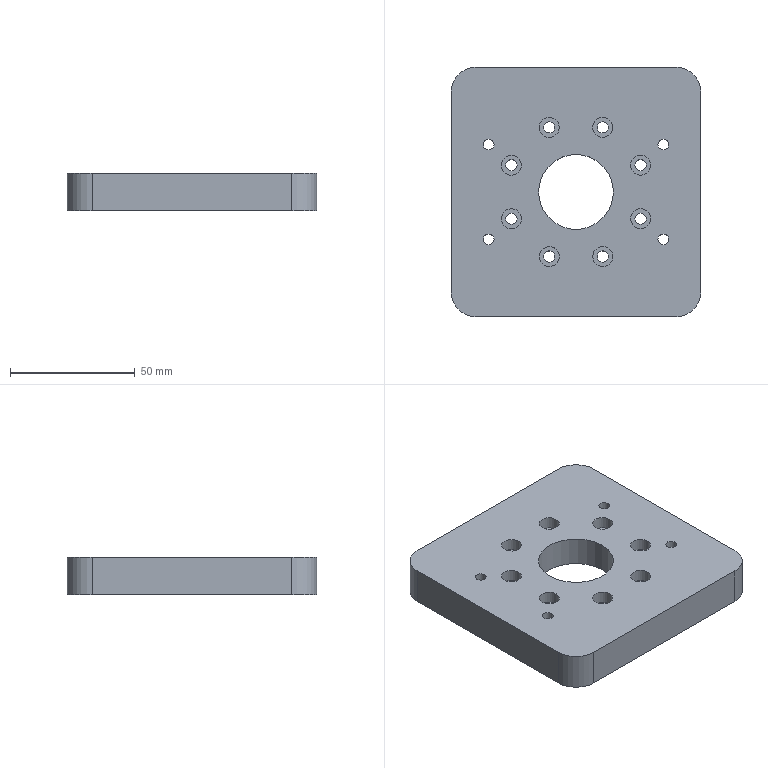NC program | NX | posted with a generic post | part box 100 x 100 x 15 mm
Lines 25 to 866 of 2115:
(ZLEVEL_PROFILE , TOOL : D10)
N48 T10 M6
N50 G54
N52 G17 G0 G90 X-53.178 Y-47.366 S9500 M3
N54 G43 Z30. H10
N56 Z1.5
N58 G94 G1 X-54.028 Y-45.669 Z1.401 F1000.
N60 X-54.754 Y-43.354 Z1.273
N62 X-55.1 Y-40.952 Z1.146
N64 Y-40. Z1.096
N66 Y0. Z-1.
N68 Y40. F3500.
N70 G2 X-40. Y55.1 R15.1
N72 G1 X40.
N74 G2 X55.1 Y40. R15.1
N76 G1 Y-40.
N78 G2 X40. Y-55.1 R15.1
N80 G1 X-40.
N82 G2 X-55.1 Y-40. R15.1
N84 G1 Y0.
N86 Y30. Z-1.072
N88 Y35. Z-1.084
N90 Y40. Z-1.096
N92 X-55.072 Y40.912 Z-1.099
N94 X-54.99 Y41.82 Z-1.101
N96 X-54.853 Y42.722 Z-1.103
N98 X-54.661 Y43.614 Z-1.105
N100 X-54.416 Y44.492 Z-1.107
N102 X-54.119 Y45.355 Z-1.11
N104 X-53.77 Y46.197 Z-1.112
N106 X-53.37 Y47.017 Z-1.114
N108 X-52.922 Y47.812 Z-1.116
N110 X-52.427 Y48.578 Z-1.118
N112 X-51.886 Y49.312 Z-1.121
N114 X-51.303 Y50.013 Z-1.123
N116 X-50.677 Y50.677 Z-1.125
N118 X-50.013 Y51.303 Z-1.127
N120 X-49.312 Y51.886 Z-1.129
N122 X-48.578 Y52.427 Z-1.132
N124 X-47.812 Y52.922 Z-1.134
N126 X-47.017 Y53.37 Z-1.136
N128 X-46.197 Y53.77 Z-1.138
N130 X-45.355 Y54.119 Z-1.14
N132 X-44.492 Y54.416 Z-1.143
N134 X-43.614 Y54.661 Z-1.145
N136 X-42.722 Y54.853 Z-1.147
N138 X-41.82 Y54.99 Z-1.149
N140 X-40.912 Y55.072 Z-1.151
N142 X-40. Y55.1 Z-1.154
N144 X30. Z-1.322
N146 X35. Z-1.334
N148 X40. Z-1.346
N150 X40.912 Y55.072 Z-1.349
N152 X41.82 Y54.99 Z-1.351
N154 X42.722 Y54.853 Z-1.353
N156 X43.614 Y54.661 Z-1.355
N158 X44.492 Y54.416 Z-1.357
N160 X45.355 Y54.119 Z-1.36
N162 X46.197 Y53.77 Z-1.362
N164 X47.017 Y53.37 Z-1.364
N166 X47.812 Y52.922 Z-1.366
N168 X48.578 Y52.427 Z-1.368
N170 X49.312 Y51.886 Z-1.371
N172 X50.013 Y51.303 Z-1.373
N174 X50.677 Y50.677 Z-1.375
N176 X51.303 Y50.013 Z-1.377
N178 X51.886 Y49.312 Z-1.379
N180 X52.427 Y48.578 Z-1.382
N182 X52.922 Y47.812 Z-1.384
N184 X53.37 Y47.017 Z-1.386
N186 X53.77 Y46.197 Z-1.388
N188 X54.119 Y45.355 Z-1.39
N190 X54.416 Y44.492 Z-1.393
N192 X54.661 Y43.614 Z-1.395
N194 X54.853 Y42.722 Z-1.397
N196 X54.99 Y41.82 Z-1.399
N198 X55.072 Y40.912 Z-1.401
N200 X55.1 Y40. Z-1.404
N202 Y-40. Z-1.596
N204 X55.072 Y-40.912 Z-1.599
N206 X54.99 Y-41.82 Z-1.601
N208 X54.853 Y-42.722 Z-1.603
N210 X54.661 Y-43.614 Z-1.605
N212 X54.416 Y-44.492 Z-1.607
N214 X54.119 Y-45.355 Z-1.61
N216 X53.77 Y-46.197 Z-1.612
N218 X53.37 Y-47.017 Z-1.614
N220 X52.922 Y-47.812 Z-1.616
N222 X52.427 Y-48.578 Z-1.618
N224 X51.886 Y-49.312 Z-1.621
N226 X51.303 Y-50.013 Z-1.623
N228 X50.677 Y-50.677 Z-1.625
N230 X50.013 Y-51.303 Z-1.627
N232 X49.312 Y-51.886 Z-1.629
N234 X48.578 Y-52.427 Z-1.632
N236 X47.812 Y-52.922 Z-1.634
N238 X47.017 Y-53.37 Z-1.636
N240 X46.197 Y-53.77 Z-1.638
N242 X45.355 Y-54.119 Z-1.64
N244 X44.492 Y-54.416 Z-1.643
N246 X43.614 Y-54.661 Z-1.645
N248 X42.722 Y-54.853 Z-1.647
N250 X41.82 Y-54.99 Z-1.649
N252 X40.912 Y-55.072 Z-1.651
N254 X40. Y-55.1 Z-1.654
N256 X-30. Z-1.822
N258 X-35. Z-1.834
N260 X-40. Z-1.846
N262 X-40.912 Y-55.072 Z-1.849
N264 X-41.82 Y-54.99 Z-1.851
N266 X-42.722 Y-54.853 Z-1.853
N268 X-43.614 Y-54.661 Z-1.855
N270 X-44.492 Y-54.416 Z-1.857
N272 X-45.355 Y-54.119 Z-1.86
N274 X-46.197 Y-53.77 Z-1.862
N276 X-47.017 Y-53.37 Z-1.864
N278 X-47.812 Y-52.922 Z-1.866
N280 X-48.578 Y-52.427 Z-1.868
N282 X-49.312 Y-51.886 Z-1.871
N284 X-50.013 Y-51.303 Z-1.873
N286 X-50.677 Y-50.677 Z-1.875
N288 X-51.303 Y-50.013 Z-1.877
N290 X-51.886 Y-49.312 Z-1.879
N292 X-52.427 Y-48.578 Z-1.882
N294 X-52.922 Y-47.812 Z-1.884
N296 X-53.37 Y-47.017 Z-1.886
N298 X-53.77 Y-46.197 Z-1.888
N300 X-54.119 Y-45.355 Z-1.89
N302 X-54.416 Y-44.492 Z-1.893
N304 X-54.661 Y-43.614 Z-1.895
N306 X-54.853 Y-42.722 Z-1.897
N308 X-54.99 Y-41.82 Z-1.899
N310 X-55.072 Y-40.912 Z-1.901
N312 X-55.1 Y-40. Z-1.904
N314 Y0. Z-2.
N316 Y30. Z-2.072
N318 Y35. Z-2.084
N320 Y40. Z-2.096
N322 X-55.072 Y40.912 Z-2.099
N324 X-54.99 Y41.82 Z-2.101
N326 X-54.853 Y42.722 Z-2.103
N328 X-54.661 Y43.614 Z-2.105
N330 X-54.416 Y44.492 Z-2.107
N332 X-54.119 Y45.355 Z-2.11
N334 X-53.77 Y46.197 Z-2.112
N336 X-53.37 Y47.017 Z-2.114
N338 X-52.922 Y47.812 Z-2.116
N340 X-52.427 Y48.578 Z-2.118
N342 X-51.886 Y49.312 Z-2.121
N344 X-51.303 Y50.013 Z-2.123
N346 X-50.677 Y50.677 Z-2.125
N348 X-50.013 Y51.303 Z-2.127
N350 X-49.312 Y51.886 Z-2.129
N352 X-48.578 Y52.427 Z-2.132
N354 X-47.812 Y52.922 Z-2.134
N356 X-47.017 Y53.37 Z-2.136
N358 X-46.197 Y53.77 Z-2.138
N360 X-45.355 Y54.119 Z-2.14
N362 X-44.492 Y54.416 Z-2.143
N364 X-43.614 Y54.661 Z-2.145
N366 X-42.722 Y54.853 Z-2.147
N368 X-41.82 Y54.99 Z-2.149
N370 X-40.912 Y55.072 Z-2.151
N372 X-40. Y55.1 Z-2.154
N374 X30. Z-2.322
N376 X35. Z-2.334
N378 X40. Z-2.346
N380 X40.912 Y55.072 Z-2.349
N382 X41.82 Y54.99 Z-2.351
N384 X42.722 Y54.853 Z-2.353
N386 X43.614 Y54.661 Z-2.355
N388 X44.492 Y54.416 Z-2.357
N390 X45.355 Y54.119 Z-2.36
N392 X46.197 Y53.77 Z-2.362
N394 X47.017 Y53.37 Z-2.364
N396 X47.812 Y52.922 Z-2.366
N398 X48.578 Y52.427 Z-2.368
N400 X49.312 Y51.886 Z-2.371
N402 X50.013 Y51.303 Z-2.373
N404 X50.677 Y50.677 Z-2.375
N406 X51.303 Y50.013 Z-2.377
N408 X51.886 Y49.312 Z-2.379
N410 X52.427 Y48.578 Z-2.382
N412 X52.922 Y47.812 Z-2.384
N414 X53.37 Y47.017 Z-2.386
N416 X53.77 Y46.197 Z-2.388
N418 X54.119 Y45.355 Z-2.39
N420 X54.416 Y44.492 Z-2.393
N422 X54.661 Y43.614 Z-2.395
N424 X54.853 Y42.722 Z-2.397
N426 X54.99 Y41.82 Z-2.399
N428 X55.072 Y40.912 Z-2.401
N430 X55.1 Y40. Z-2.404
N432 Y-40. Z-2.596
N434 X55.072 Y-40.912 Z-2.599
N436 X54.99 Y-41.82 Z-2.601
N438 X54.853 Y-42.722 Z-2.603
N440 X54.661 Y-43.614 Z-2.605
N442 X54.416 Y-44.492 Z-2.607
N444 X54.119 Y-45.355 Z-2.61
N446 X53.77 Y-46.197 Z-2.612
N448 X53.37 Y-47.017 Z-2.614
N450 X52.922 Y-47.812 Z-2.616
N452 X52.427 Y-48.578 Z-2.618
N454 X51.886 Y-49.312 Z-2.621
N456 X51.303 Y-50.013 Z-2.623
N458 X50.677 Y-50.677 Z-2.625
N460 X50.013 Y-51.303 Z-2.627
N462 X49.312 Y-51.886 Z-2.629
N464 X48.578 Y-52.427 Z-2.632
N466 X47.812 Y-52.922 Z-2.634
N468 X47.017 Y-53.37 Z-2.636
N470 X46.197 Y-53.77 Z-2.638
N472 X45.355 Y-54.119 Z-2.64
N474 X44.492 Y-54.416 Z-2.643
N476 X43.614 Y-54.661 Z-2.645
N478 X42.722 Y-54.853 Z-2.647
N480 X41.82 Y-54.99 Z-2.649
N482 X40.912 Y-55.072 Z-2.651
N484 X40. Y-55.1 Z-2.654
N486 X-30. Z-2.822
N488 X-35. Z-2.834
N490 X-40. Z-2.846
N492 X-40.912 Y-55.072 Z-2.849
N494 X-41.82 Y-54.99 Z-2.851
N496 X-42.722 Y-54.853 Z-2.853
N498 X-43.614 Y-54.661 Z-2.855
N500 X-44.492 Y-54.416 Z-2.857
N502 X-45.355 Y-54.119 Z-2.86
N504 X-46.197 Y-53.77 Z-2.862
N506 X-47.017 Y-53.37 Z-2.864
N508 X-47.812 Y-52.922 Z-2.866
N510 X-48.578 Y-52.427 Z-2.868
N512 X-49.312 Y-51.886 Z-2.871
N514 X-50.013 Y-51.303 Z-2.873
N516 X-50.677 Y-50.677 Z-2.875
N518 X-51.303 Y-50.013 Z-2.877
N520 X-51.886 Y-49.312 Z-2.879
N522 X-52.427 Y-48.578 Z-2.882
N524 X-52.922 Y-47.812 Z-2.884
N526 X-53.37 Y-47.017 Z-2.886
N528 X-53.77 Y-46.197 Z-2.888
N530 X-54.119 Y-45.355 Z-2.89
N532 X-54.416 Y-44.492 Z-2.893
N534 X-54.661 Y-43.614 Z-2.895
N536 X-54.853 Y-42.722 Z-2.897
N538 X-54.99 Y-41.82 Z-2.899
N540 X-55.072 Y-40.912 Z-2.901
N542 X-55.1 Y-40. Z-2.904
N544 Y0. Z-3.
N546 Y30. Z-3.072
N548 Y35. Z-3.084
N550 Y40. Z-3.096
N552 X-55.072 Y40.912 Z-3.099
N554 X-54.99 Y41.82 Z-3.101
N556 X-54.853 Y42.722 Z-3.103
N558 X-54.661 Y43.614 Z-3.105
N560 X-54.416 Y44.492 Z-3.107
N562 X-54.119 Y45.355 Z-3.11
N564 X-53.77 Y46.197 Z-3.112
N566 X-53.37 Y47.017 Z-3.114
N568 X-52.922 Y47.812 Z-3.116
N570 X-52.427 Y48.578 Z-3.118
N572 X-51.886 Y49.312 Z-3.121
N574 X-51.303 Y50.013 Z-3.123
N576 X-50.677 Y50.677 Z-3.125
N578 X-50.013 Y51.303 Z-3.127
N580 X-49.312 Y51.886 Z-3.129
N582 X-48.578 Y52.427 Z-3.132
N584 X-47.812 Y52.922 Z-3.134
N586 X-47.017 Y53.37 Z-3.136
N588 X-46.197 Y53.77 Z-3.138
N590 X-45.355 Y54.119 Z-3.14
N592 X-44.492 Y54.416 Z-3.143
N594 X-43.614 Y54.661 Z-3.145
N596 X-42.722 Y54.853 Z-3.147
N598 X-41.82 Y54.99 Z-3.149
N600 X-40.912 Y55.072 Z-3.151
N602 X-40. Y55.1 Z-3.154
N604 X30. Z-3.322
N606 X35. Z-3.334
N608 X40. Z-3.346
N610 X40.912 Y55.072 Z-3.349
N612 X41.82 Y54.99 Z-3.351
N614 X42.722 Y54.853 Z-3.353
N616 X43.614 Y54.661 Z-3.355
N618 X44.492 Y54.416 Z-3.357
N620 X45.355 Y54.119 Z-3.36
N622 X46.197 Y53.77 Z-3.362
N624 X47.017 Y53.37 Z-3.364
N626 X47.812 Y52.922 Z-3.366
N628 X48.578 Y52.427 Z-3.368
N630 X49.312 Y51.886 Z-3.371
N632 X50.013 Y51.303 Z-3.373
N634 X50.677 Y50.677 Z-3.375
N636 X51.303 Y50.013 Z-3.377
N638 X51.886 Y49.312 Z-3.379
N640 X52.427 Y48.578 Z-3.382
N642 X52.922 Y47.812 Z-3.384
N644 X53.37 Y47.017 Z-3.386
N646 X53.77 Y46.197 Z-3.388
N648 X54.119 Y45.355 Z-3.39
N650 X54.416 Y44.492 Z-3.393
N652 X54.661 Y43.614 Z-3.395
N654 X54.853 Y42.722 Z-3.397
N656 X54.99 Y41.82 Z-3.399
N658 X55.072 Y40.912 Z-3.401
N660 X55.1 Y40. Z-3.404
N662 Y-40. Z-3.596
N664 X55.072 Y-40.912 Z-3.599
N666 X54.99 Y-41.82 Z-3.601
N668 X54.853 Y-42.722 Z-3.603
N670 X54.661 Y-43.614 Z-3.605
N672 X54.416 Y-44.492 Z-3.607
N674 X54.119 Y-45.355 Z-3.61
N676 X53.77 Y-46.197 Z-3.612
N678 X53.37 Y-47.017 Z-3.614
N680 X52.922 Y-47.812 Z-3.616
N682 X52.427 Y-48.578 Z-3.618
N684 X51.886 Y-49.312 Z-3.621
N686 X51.303 Y-50.013 Z-3.623
N688 X50.677 Y-50.677 Z-3.625
N690 X50.013 Y-51.303 Z-3.627
N692 X49.312 Y-51.886 Z-3.629
N694 X48.578 Y-52.427 Z-3.632
N696 X47.812 Y-52.922 Z-3.634
N698 X47.017 Y-53.37 Z-3.636
N700 X46.197 Y-53.77 Z-3.638
N702 X45.355 Y-54.119 Z-3.64
N704 X44.492 Y-54.416 Z-3.643
N706 X43.614 Y-54.661 Z-3.645
N708 X42.722 Y-54.853 Z-3.647
N710 X41.82 Y-54.99 Z-3.649
N712 X40.912 Y-55.072 Z-3.651
N714 X40. Y-55.1 Z-3.654
N716 X-30. Z-3.822
N718 X-35. Z-3.834
N720 X-40. Z-3.846
N722 X-40.912 Y-55.072 Z-3.849
N724 X-41.82 Y-54.99 Z-3.851
N726 X-42.722 Y-54.853 Z-3.853
N728 X-43.614 Y-54.661 Z-3.855
N730 X-44.492 Y-54.416 Z-3.857
N732 X-45.355 Y-54.119 Z-3.86
N734 X-46.197 Y-53.77 Z-3.862
N736 X-47.017 Y-53.37 Z-3.864
N738 X-47.812 Y-52.922 Z-3.866
N740 X-48.578 Y-52.427 Z-3.868
N742 X-49.312 Y-51.886 Z-3.871
N744 X-50.013 Y-51.303 Z-3.873
N746 X-50.677 Y-50.677 Z-3.875
N748 X-51.303 Y-50.013 Z-3.877
N750 X-51.886 Y-49.312 Z-3.879
N752 X-52.427 Y-48.578 Z-3.882
N754 X-52.922 Y-47.812 Z-3.884
N756 X-53.37 Y-47.017 Z-3.886
N758 X-53.77 Y-46.197 Z-3.888
N760 X-54.119 Y-45.355 Z-3.89
N762 X-54.416 Y-44.492 Z-3.893
N764 X-54.661 Y-43.614 Z-3.895
N766 X-54.853 Y-42.722 Z-3.897
N768 X-54.99 Y-41.82 Z-3.899
N770 X-55.072 Y-40.912 Z-3.901
N772 X-55.1 Y-40. Z-3.904
N774 Y0. Z-4.
N776 Y30. Z-4.072
N778 Y35. Z-4.084
N780 Y40. Z-4.096
N782 X-55.072 Y40.912 Z-4.099
N784 X-54.99 Y41.82 Z-4.101
N786 X-54.853 Y42.722 Z-4.103
N788 X-54.661 Y43.614 Z-4.105
N790 X-54.416 Y44.492 Z-4.107
N792 X-54.119 Y45.355 Z-4.11
N794 X-53.77 Y46.197 Z-4.112
N796 X-53.37 Y47.017 Z-4.114
N798 X-52.922 Y47.812 Z-4.116
N800 X-52.427 Y48.578 Z-4.118
N802 X-51.886 Y49.312 Z-4.121
N804 X-51.303 Y50.013 Z-4.123
N806 X-50.677 Y50.677 Z-4.125
N808 X-50.013 Y51.303 Z-4.127
N810 X-49.312 Y51.886 Z-4.129
N812 X-48.578 Y52.427 Z-4.132
N814 X-47.812 Y52.922 Z-4.134
N816 X-47.017 Y53.37 Z-4.136
N818 X-46.197 Y53.77 Z-4.138
N820 X-45.355 Y54.119 Z-4.14
N822 X-44.492 Y54.416 Z-4.143
N824 X-43.614 Y54.661 Z-4.145
N826 X-42.722 Y54.853 Z-4.147
N828 X-41.82 Y54.99 Z-4.149
N830 X-40.912 Y55.072 Z-4.151
N832 X-40. Y55.1 Z-4.154
N834 X30. Z-4.322
N836 X35. Z-4.334
N838 X40. Z-4.346
N840 X40.912 Y55.072 Z-4.349
N842 X41.82 Y54.99 Z-4.351
N844 X42.722 Y54.853 Z-4.353
N846 X43.614 Y54.661 Z-4.355
N848 X44.492 Y54.416 Z-4.357
N850 X45.355 Y54.119 Z-4.36
N852 X46.197 Y53.77 Z-4.362
N854 X47.017 Y53.37 Z-4.364
N856 X47.812 Y52.922 Z-4.366
N858 X48.578 Y52.427 Z-4.368
N860 X49.312 Y51.886 Z-4.371
N862 X50.013 Y51.303 Z-4.373
N864 X50.677 Y50.677 Z-4.375
N866 X51.303 Y50.013 Z-4.377
N868 X51.886 Y49.312 Z-4.379
N870 X52.427 Y48.578 Z-4.382
N872 X52.922 Y47.812 Z-4.384
N874 X53.37 Y47.017 Z-4.386
N876 X53.77 Y46.197 Z-4.388
N878 X54.119 Y45.355 Z-4.39
N880 X54.416 Y44.492 Z-4.393
N882 X54.661 Y43.614 Z-4.395
N884 X54.853 Y42.722 Z-4.397
N886 X54.99 Y41.82 Z-4.399
N888 X55.072 Y40.912 Z-4.401
N890 X55.1 Y40. Z-4.404
N892 Y-40. Z-4.596
N894 X55.072 Y-40.912 Z-4.599
N896 X54.99 Y-41.82 Z-4.601
N898 X54.853 Y-42.722 Z-4.603
N900 X54.661 Y-43.614 Z-4.605
N902 X54.416 Y-44.492 Z-4.607
N904 X54.119 Y-45.355 Z-4.61
N906 X53.77 Y-46.197 Z-4.612
N908 X53.37 Y-47.017 Z-4.614
N910 X52.922 Y-47.812 Z-4.616
N912 X52.427 Y-48.578 Z-4.618
N914 X51.886 Y-49.312 Z-4.621
N916 X51.303 Y-50.013 Z-4.623
N918 X50.677 Y-50.677 Z-4.625
N920 X50.013 Y-51.303 Z-4.627
N922 X49.312 Y-51.886 Z-4.629
N924 X48.578 Y-52.427 Z-4.632
N926 X47.812 Y-52.922 Z-4.634
N928 X47.017 Y-53.37 Z-4.636
N930 X46.197 Y-53.77 Z-4.638
N932 X45.355 Y-54.119 Z-4.64
N934 X44.492 Y-54.416 Z-4.643
N936 X43.614 Y-54.661 Z-4.645
N938 X42.722 Y-54.853 Z-4.647
N940 X41.82 Y-54.99 Z-4.649
N942 X40.912 Y-55.072 Z-4.651
N944 X40. Y-55.1 Z-4.654
N946 X-30. Z-4.822
N948 X-35. Z-4.834
N950 X-40. Z-4.846
N952 X-40.912 Y-55.072 Z-4.849
N954 X-41.82 Y-54.99 Z-4.851
N956 X-42.722 Y-54.853 Z-4.853
N958 X-43.614 Y-54.661 Z-4.855
N960 X-44.492 Y-54.416 Z-4.857
N962 X-45.355 Y-54.119 Z-4.86
N964 X-46.197 Y-53.77 Z-4.862
N966 X-47.017 Y-53.37 Z-4.864
N968 X-47.812 Y-52.922 Z-4.866
N970 X-48.578 Y-52.427 Z-4.868
N972 X-49.312 Y-51.886 Z-4.871
N974 X-50.013 Y-51.303 Z-4.873
N976 X-50.677 Y-50.677 Z-4.875
N978 X-51.303 Y-50.013 Z-4.877
N980 X-51.886 Y-49.312 Z-4.879
N982 X-52.427 Y-48.578 Z-4.882
N984 X-52.922 Y-47.812 Z-4.884
N986 X-53.37 Y-47.017 Z-4.886
N988 X-53.77 Y-46.197 Z-4.888
N990 X-54.119 Y-45.355 Z-4.89
N992 X-54.416 Y-44.492 Z-4.893
N994 X-54.661 Y-43.614 Z-4.895
N996 X-54.853 Y-42.722 Z-4.897
N998 X-54.99 Y-41.82 Z-4.899
N1000 X-55.072 Y-40.912 Z-4.901
N1002 X-55.1 Y-40. Z-4.904
N1004 Y0. Z-5.
N1006 Y30. Z-5.072
N1008 Y35. Z-5.084
N1010 Y40. Z-5.096
N1012 X-55.072 Y40.912 Z-5.099
N1014 X-54.99 Y41.82 Z-5.101
N1016 X-54.853 Y42.722 Z-5.103
N1018 X-54.661 Y43.614 Z-5.105
N1020 X-54.416 Y44.492 Z-5.107
N1022 X-54.119 Y45.355 Z-5.11
N1024 X-53.77 Y46.197 Z-5.112
N1026 X-53.37 Y47.017 Z-5.114
N1028 X-52.922 Y47.812 Z-5.116
N1030 X-52.427 Y48.578 Z-5.118
N1032 X-51.886 Y49.312 Z-5.121
N1034 X-51.303 Y50.013 Z-5.123
N1036 X-50.677 Y50.677 Z-5.125
N1038 X-50.013 Y51.303 Z-5.127
N1040 X-49.312 Y51.886 Z-5.129
N1042 X-48.578 Y52.427 Z-5.132
N1044 X-47.812 Y52.922 Z-5.134
N1046 X-47.017 Y53.37 Z-5.136
N1048 X-46.197 Y53.77 Z-5.138
N1050 X-45.355 Y54.119 Z-5.14
N1052 X-44.492 Y54.416 Z-5.143
N1054 X-43.614 Y54.661 Z-5.145
N1056 X-42.722 Y54.853 Z-5.147
N1058 X-41.82 Y54.99 Z-5.149
N1060 X-40.912 Y55.072 Z-5.151
N1062 X-40. Y55.1 Z-5.154
N1064 X30. Z-5.322
N1066 X35. Z-5.334
N1068 X40. Z-5.346
N1070 X40.912 Y55.072 Z-5.349
N1072 X41.82 Y54.99 Z-5.351
N1074 X42.722 Y54.853 Z-5.353
N1076 X43.614 Y54.661 Z-5.355
N1078 X44.492 Y54.416 Z-5.357
N1080 X45.355 Y54.119 Z-5.36
N1082 X46.197 Y53.77 Z-5.362
N1084 X47.017 Y53.37 Z-5.364
N1086 X47.812 Y52.922 Z-5.366
N1088 X48.578 Y52.427 Z-5.368
N1090 X49.312 Y51.886 Z-5.371
N1092 X50.013 Y51.303 Z-5.373
N1094 X50.677 Y50.677 Z-5.375
N1096 X51.303 Y50.013 Z-5.377
N1098 X51.886 Y49.312 Z-5.379
N1100 X52.427 Y48.578 Z-5.382
N1102 X52.922 Y47.812 Z-5.384
N1104 X53.37 Y47.017 Z-5.386
N1106 X53.77 Y46.197 Z-5.388
N1108 X54.119 Y45.355 Z-5.39
N1110 X54.416 Y44.492 Z-5.393
N1112 X54.661 Y43.614 Z-5.395
N1114 X54.853 Y42.722 Z-5.397
N1116 X54.99 Y41.82 Z-5.399
N1118 X55.072 Y40.912 Z-5.401
N1120 X55.1 Y40. Z-5.404
N1122 Y-40. Z-5.596
N1124 X55.072 Y-40.912 Z-5.599
N1126 X54.99 Y-41.82 Z-5.601
N1128 X54.853 Y-42.722 Z-5.603
N1130 X54.661 Y-43.614 Z-5.605
N1132 X54.416 Y-44.492 Z-5.607
N1134 X54.119 Y-45.355 Z-5.61
N1136 X53.77 Y-46.197 Z-5.612
N1138 X53.37 Y-47.017 Z-5.614
N1140 X52.922 Y-47.812 Z-5.616
N1142 X52.427 Y-48.578 Z-5.618
N1144 X51.886 Y-49.312 Z-5.621
N1146 X51.303 Y-50.013 Z-5.623
N1148 X50.677 Y-50.677 Z-5.625
N1150 X50.013 Y-51.303 Z-5.627
N1152 X49.312 Y-51.886 Z-5.629
N1154 X48.578 Y-52.427 Z-5.632
N1156 X47.812 Y-52.922 Z-5.634
N1158 X47.017 Y-53.37 Z-5.636
N1160 X46.197 Y-53.77 Z-5.638
N1162 X45.355 Y-54.119 Z-5.64
N1164 X44.492 Y-54.416 Z-5.643
N1166 X43.614 Y-54.661 Z-5.645
N1168 X42.722 Y-54.853 Z-5.647
N1170 X41.82 Y-54.99 Z-5.649
N1172 X40.912 Y-55.072 Z-5.651
N1174 X40. Y-55.1 Z-5.654
N1176 X-30. Z-5.822
N1178 X-35. Z-5.834
N1180 X-40. Z-5.846
N1182 X-40.912 Y-55.072 Z-5.849
N1184 X-41.82 Y-54.99 Z-5.851
N1186 X-42.722 Y-54.853 Z-5.853
N1188 X-43.614 Y-54.661 Z-5.855
N1190 X-44.492 Y-54.416 Z-5.857
N1192 X-45.355 Y-54.119 Z-5.86
N1194 X-46.197 Y-53.77 Z-5.862
N1196 X-47.017 Y-53.37 Z-5.864
N1198 X-47.812 Y-52.922 Z-5.866
N1200 X-48.578 Y-52.427 Z-5.868
N1202 X-49.312 Y-51.886 Z-5.871
N1204 X-50.013 Y-51.303 Z-5.873
N1206 X-50.677 Y-50.677 Z-5.875
N1208 X-51.303 Y-50.013 Z-5.877
N1210 X-51.886 Y-49.312 Z-5.879
N1212 X-52.427 Y-48.578 Z-5.882
N1214 X-52.922 Y-47.812 Z-5.884
N1216 X-53.37 Y-47.017 Z-5.886
N1218 X-53.77 Y-46.197 Z-5.888
N1220 X-54.119 Y-45.355 Z-5.89
N1222 X-54.416 Y-44.492 Z-5.893
N1224 X-54.661 Y-43.614 Z-5.895
N1226 X-54.853 Y-42.722 Z-5.897
N1228 X-54.99 Y-41.82 Z-5.899
N1230 X-55.072 Y-40.912 Z-5.901
N1232 X-55.1 Y-40. Z-5.904
N1234 Y0. Z-6.
N1236 Y30. Z-6.072
N1238 Y35. Z-6.084
N1240 Y40. Z-6.096
N1242 X-55.072 Y40.912 Z-6.099
N1244 X-54.99 Y41.82 Z-6.101
N1246 X-54.853 Y42.722 Z-6.103
N1248 X-54.661 Y43.614 Z-6.105
N1250 X-54.416 Y44.492 Z-6.107
N1252 X-54.119 Y45.355 Z-6.11
N1254 X-53.77 Y46.197 Z-6.112
N1256 X-53.37 Y47.017 Z-6.114
N1258 X-52.922 Y47.812 Z-6.116
N1260 X-52.427 Y48.578 Z-6.118
N1262 X-51.886 Y49.312 Z-6.121
N1264 X-51.303 Y50.013 Z-6.123
N1266 X-50.677 Y50.677 Z-6.125
N1268 X-50.013 Y51.303 Z-6.127
N1270 X-49.312 Y51.886 Z-6.129
N1272 X-48.578 Y52.427 Z-6.132
N1274 X-47.812 Y52.922 Z-6.134
N1276 X-47.017 Y53.37 Z-6.136
N1278 X-46.197 Y53.77 Z-6.138
N1280 X-45.355 Y54.119 Z-6.14
N1282 X-44.492 Y54.416 Z-6.143
N1284 X-43.614 Y54.661 Z-6.145
N1286 X-42.722 Y54.853 Z-6.147
N1288 X-41.82 Y54.99 Z-6.149
N1290 X-40.912 Y55.072 Z-6.151
N1292 X-40. Y55.1 Z-6.154
N1294 X30. Z-6.322
N1296 X35. Z-6.334
N1298 X40. Z-6.346
N1300 X40.912 Y55.072 Z-6.349
N1302 X41.82 Y54.99 Z-6.351
N1304 X42.722 Y54.853 Z-6.353
N1306 X43.614 Y54.661 Z-6.355
N1308 X44.492 Y54.416 Z-6.357
N1310 X45.355 Y54.119 Z-6.36
N1312 X46.197 Y53.77 Z-6.362
N1314 X47.017 Y53.37 Z-6.364
N1316 X47.812 Y52.922 Z-6.366
N1318 X48.578 Y52.427 Z-6.368
N1320 X49.312 Y51.886 Z-6.371
N1322 X50.013 Y51.303 Z-6.373
N1324 X50.677 Y50.677 Z-6.375
N1326 X51.303 Y50.013 Z-6.377
N1328 X51.886 Y49.312 Z-6.379
N1330 X52.427 Y48.578 Z-6.382
N1332 X52.922 Y47.812 Z-6.384
N1334 X53.37 Y47.017 Z-6.386
N1336 X53.77 Y46.197 Z-6.388
N1338 X54.119 Y45.355 Z-6.39
N1340 X54.416 Y44.492 Z-6.393
N1342 X54.661 Y43.614 Z-6.395
N1344 X54.853 Y42.722 Z-6.397
N1346 X54.99 Y41.82 Z-6.399
N1348 X55.072 Y40.912 Z-6.401
N1350 X55.1 Y40. Z-6.404
N1352 Y-40. Z-6.596
N1354 X55.072 Y-40.912 Z-6.599
N1356 X54.99 Y-41.82 Z-6.601
N1358 X54.853 Y-42.722 Z-6.603
N1360 X54.661 Y-43.614 Z-6.605
N1362 X54.416 Y-44.492 Z-6.607
N1364 X54.119 Y-45.355 Z-6.61
N1366 X53.77 Y-46.197 Z-6.612
N1368 X53.37 Y-47.017 Z-6.614
N1370 X52.922 Y-47.812 Z-6.616
N1372 X52.427 Y-48.578 Z-6.618
N1374 X51.886 Y-49.312 Z-6.621
N1376 X51.303 Y-50.013 Z-6.623
N1378 X50.677 Y-50.677 Z-6.625
N1380 X50.013 Y-51.303 Z-6.627
N1382 X49.312 Y-51.886 Z-6.629
N1384 X48.578 Y-52.427 Z-6.632
N1386 X47.812 Y-52.922 Z-6.634
N1388 X47.017 Y-53.37 Z-6.636
N1390 X46.197 Y-53.77 Z-6.638
N1392 X45.355 Y-54.119 Z-6.64
N1394 X44.492 Y-54.416 Z-6.643
N1396 X43.614 Y-54.661 Z-6.645
N1398 X42.722 Y-54.853 Z-6.647
N1400 X41.82 Y-54.99 Z-6.649
N1402 X40.912 Y-55.072 Z-6.651
N1404 X40. Y-55.1 Z-6.654
N1406 X-30. Z-6.822
N1408 X-35. Z-6.834
N1410 X-40. Z-6.846
N1412 X-40.912 Y-55.072 Z-6.849
N1414 X-41.82 Y-54.99 Z-6.851
N1416 X-42.722 Y-54.853 Z-6.853
N1418 X-43.614 Y-54.661 Z-6.855
N1420 X-44.492 Y-54.416 Z-6.857
N1422 X-45.355 Y-54.119 Z-6.86
N1424 X-46.197 Y-53.77 Z-6.862
N1426 X-47.017 Y-53.37 Z-6.864
N1428 X-47.812 Y-52.922 Z-6.866
N1430 X-48.578 Y-52.427 Z-6.868
N1432 X-49.312 Y-51.886 Z-6.871
N1434 X-50.013 Y-51.303 Z-6.873
N1436 X-50.677 Y-50.677 Z-6.875
N1438 X-51.303 Y-50.013 Z-6.877
N1440 X-51.886 Y-49.312 Z-6.879
N1442 X-52.427 Y-48.578 Z-6.882
N1444 X-52.922 Y-47.812 Z-6.884
N1446 X-53.37 Y-47.017 Z-6.886
N1448 X-53.77 Y-46.197 Z-6.888
N1450 X-54.119 Y-45.355 Z-6.89
N1452 X-54.416 Y-44.492 Z-6.893
N1454 X-54.661 Y-43.614 Z-6.895
N1456 X-54.853 Y-42.722 Z-6.897
N1458 X-54.99 Y-41.82 Z-6.899
N1460 X-55.072 Y-40.912 Z-6.901
N1462 X-55.1 Y-40. Z-6.904
N1464 Y0. Z-7.
N1466 Y30. Z-7.072
N1468 Y35. Z-7.084
N1470 Y40. Z-7.096
N1472 X-55.072 Y40.912 Z-7.099
N1474 X-54.99 Y41.82 Z-7.101
N1476 X-54.853 Y42.722 Z-7.103
N1478 X-54.661 Y43.614 Z-7.105
N1480 X-54.416 Y44.492 Z-7.107
N1482 X-54.119 Y45.355 Z-7.11
N1484 X-53.77 Y46.197 Z-7.112
N1486 X-53.37 Y47.017 Z-7.114
N1488 X-52.922 Y47.812 Z-7.116
N1490 X-52.427 Y48.578 Z-7.118
N1492 X-51.886 Y49.312 Z-7.121
N1494 X-51.303 Y50.013 Z-7.123
N1496 X-50.677 Y50.677 Z-7.125
N1498 X-50.013 Y51.303 Z-7.127
N1500 X-49.312 Y51.886 Z-7.129
N1502 X-48.578 Y52.427 Z-7.132
N1504 X-47.812 Y52.922 Z-7.134
N1506 X-47.017 Y53.37 Z-7.136
N1508 X-46.197 Y53.77 Z-7.138
N1510 X-45.355 Y54.119 Z-7.14
N1512 X-44.492 Y54.416 Z-7.143
N1514 X-43.614 Y54.661 Z-7.145
N1516 X-42.722 Y54.853 Z-7.147
N1518 X-41.82 Y54.99 Z-7.149
N1520 X-40.912 Y55.072 Z-7.151
N1522 X-40. Y55.1 Z-7.154
N1524 X30. Z-7.322
N1526 X35. Z-7.334
N1528 X40. Z-7.346
N1530 X40.912 Y55.072 Z-7.349
N1532 X41.82 Y54.99 Z-7.351
N1534 X42.722 Y54.853 Z-7.353
N1536 X43.614 Y54.661 Z-7.355
N1538 X44.492 Y54.416 Z-7.357
N1540 X45.355 Y54.119 Z-7.36
N1542 X46.197 Y53.77 Z-7.362
N1544 X47.017 Y53.37 Z-7.364
N1546 X47.812 Y52.922 Z-7.366
N1548 X48.578 Y52.427 Z-7.368
N1550 X49.312 Y51.886 Z-7.371
N1552 X50.013 Y51.303 Z-7.373
N1554 X50.677 Y50.677 Z-7.375
N1556 X51.303 Y50.013 Z-7.377
N1558 X51.886 Y49.312 Z-7.379
N1560 X52.427 Y48.578 Z-7.382
N1562 X52.922 Y47.812 Z-7.384
N1564 X53.37 Y47.017 Z-7.386
N1566 X53.77 Y46.197 Z-7.388
N1568 X54.119 Y45.355 Z-7.39
N1570 X54.416 Y44.492 Z-7.393
N1572 X54.661 Y43.614 Z-7.395
N1574 X54.853 Y42.722 Z-7.397
N1576 X54.99 Y41.82 Z-7.399
N1578 X55.072 Y40.912 Z-7.401
N1580 X55.1 Y40. Z-7.404
N1582 Y-40. Z-7.596
N1584 X55.072 Y-40.912 Z-7.599
N1586 X54.99 Y-41.82 Z-7.601
N1588 X54.853 Y-42.722 Z-7.603
N1590 X54.661 Y-43.614 Z-7.605
N1592 X54.416 Y-44.492 Z-7.607
N1594 X54.119 Y-45.355 Z-7.61
N1596 X53.77 Y-46.197 Z-7.612
N1598 X53.37 Y-47.017 Z-7.614
N1600 X52.922 Y-47.812 Z-7.616
N1602 X52.427 Y-48.578 Z-7.618
N1604 X51.886 Y-49.312 Z-7.621
N1606 X51.303 Y-50.013 Z-7.623
N1608 X50.677 Y-50.677 Z-7.625
N1610 X50.013 Y-51.303 Z-7.627
N1612 X49.312 Y-51.886 Z-7.629
N1614 X48.578 Y-52.427 Z-7.632
N1616 X47.812 Y-52.922 Z-7.634
N1618 X47.017 Y-53.37 Z-7.636
N1620 X46.197 Y-53.77 Z-7.638
N1622 X45.355 Y-54.119 Z-7.64
N1624 X44.492 Y-54.416 Z-7.643
N1626 X43.614 Y-54.661 Z-7.645
N1628 X42.722 Y-54.853 Z-7.647
N1630 X41.82 Y-54.99 Z-7.649
N1632 X40.912 Y-55.072 Z-7.651
N1634 X40. Y-55.1 Z-7.654
N1636 X-30. Z-7.822
N1638 X-35. Z-7.834
N1640 X-40. Z-7.846
N1642 X-40.912 Y-55.072 Z-7.849
N1644 X-41.82 Y-54.99 Z-7.851
N1646 X-42.722 Y-54.853 Z-7.853
N1648 X-43.614 Y-54.661 Z-7.855
N1650 X-44.492 Y-54.416 Z-7.857
N1652 X-45.355 Y-54.119 Z-7.86
N1654 X-46.197 Y-53.77 Z-7.862
N1656 X-47.017 Y-53.37 Z-7.864
N1658 X-47.812 Y-52.922 Z-7.866
N1660 X-48.578 Y-52.427 Z-7.868
N1662 X-49.312 Y-51.886 Z-7.871
N1664 X-50.013 Y-51.303 Z-7.873
N1666 X-50.677 Y-50.677 Z-7.875
N1668 X-51.303 Y-50.013 Z-7.877
N1670 X-51.886 Y-49.312 Z-7.879
N1672 X-52.427 Y-48.578 Z-7.882
N1674 X-52.922 Y-47.812 Z-7.884
N1676 X-53.37 Y-47.017 Z-7.886
N1678 X-53.77 Y-46.197 Z-7.888
N1680 X-54.119 Y-45.355 Z-7.89
N1682 X-54.416 Y-44.492 Z-7.893
N1684 X-54.661 Y-43.614 Z-7.895
N1686 X-54.853 Y-42.722 Z-7.897
N1688 X-54.99 Y-41.82 Z-7.899
N1690 X-55.072 Y-40.912 Z-7.901
N1692 X-55.1 Y-40. Z-7.904
N1694 Y0. Z-8.
N1696 Y30. Z-8.072
N1698 Y35. Z-8.084
N1700 Y40. Z-8.096
N1702 X-55.072 Y40.912 Z-8.099
N1704 X-54.99 Y41.82 Z-8.101
N1706 X-54.853 Y42.722 Z-8.103
N1708 X-54.661 Y43.614 Z-8.105
N1710 X-54.416 Y44.492 Z-8.107
N1712 X-54.119 Y45.355 Z-8.11
N1714 X-53.77 Y46.197 Z-8.112
N1716 X-53.37 Y47.017 Z-8.114
N1718 X-52.922 Y47.812 Z-8.116
N1720 X-52.427 Y48.578 Z-8.118
N1722 X-51.886 Y49.312 Z-8.121
N1724 X-51.303 Y50.013 Z-8.123